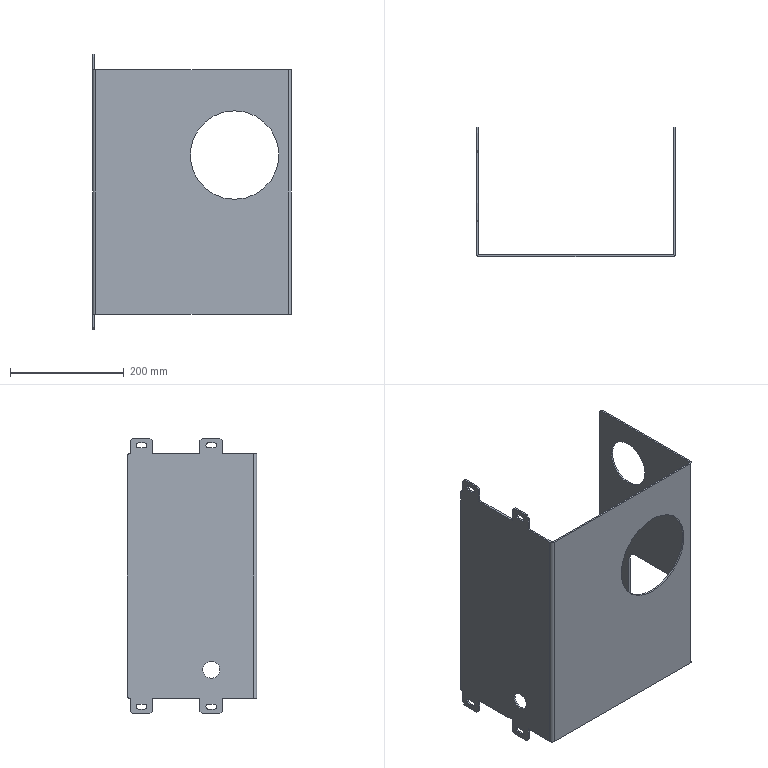Part | SolidWorks | features ICE 5, Chamfer 1, Fillet 1, FlatPattern 1, SMBaseFlange 1, SheetMetal 1, UnFold 1 | 1 solid | 80 faces | box 350 x 228 x 486 mm | volume 915789 mm3 | plane 54 | cylinder 26 | commonest cylinder face diameters 9 x8 6 x4 32 x4 5 x2 11 x2 30 x2